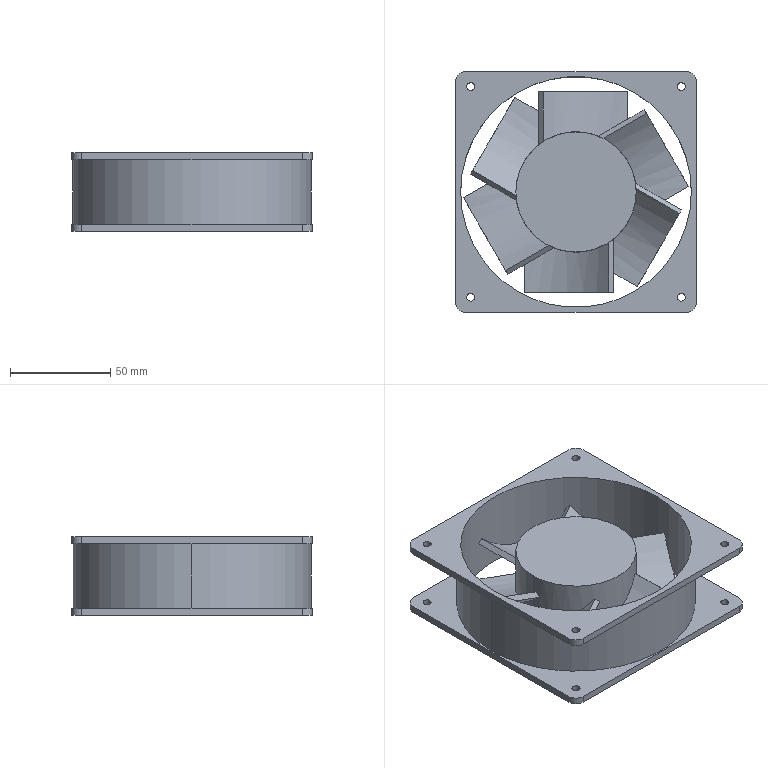Part | STEP file | Label: fan 105×105 | 2 solids | 74 faces | box 120 x 120 x 39 mm | volume 155922 mm3 | plane 32 | cylinder 30 | spline 12 | commonest cylinder face diameters 4 x16 10 x8 60 x2 115 x2 119 x2